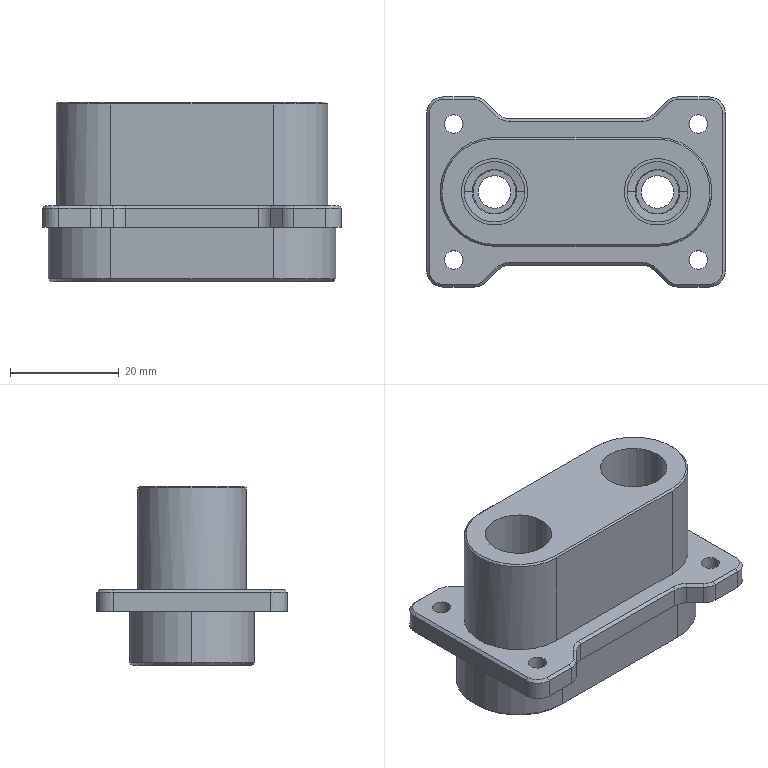NC program | NX | posted with a generic post | part box 55 x 35 x 33 mm
Whole program:
N10 G17 G21 G94 G90
(PLANAR_MILL_6 , TOOL : D6开粗)
N12 T02 M6
N14 G54
N16 G17 G0 G90 X-0.05 Y-1.639 S6500 M3
N18 G43 Z30. H2
N20 Z1.
N22 G94 G1 Y-15.051 Z0.297 F2000.
N24 X0.05 Z0.292
N26 Y-0.001 Z-0.497
N28 Y14.999
N30 X0. Y15.074
N32 X-0.05 Y14.999
N34 Y-15.001
N36 X0. Y-15.076
N38 X0.05 Y-15.001
N40 Y-0.001
N42 X4.25
N44 Y14.999
N46 G3 X0. Y19.249 R4.25
N48 X-4.25 Y14.999 R4.25
N50 G1 Y-15.001
N52 G3 X0. Y-19.251 R4.25
N54 X4.25 Y-15.001 R4.25
N56 G1 Y-0.001
N58 X8.45
N60 Y14.999
N62 G3 X0. Y23.449 R8.45
N64 X-8.45 Y14.999 R8.45
N66 G1 Y-15.001
N68 G3 X0. Y-23.451 R8.45
N70 X8.45 Y-15.001 R8.45
N72 G1 Y-0.001
N74 Z0.503
N76 G0 Z30.
N78 X-0.05 Y-1.639
N80 Z0.503
N82 G1 Y-15.051 Z-0.2
N84 X0.05 Z-0.205
N86 Y-0.001 Z-0.994
N88 Y14.999
N90 X0. Y15.074
N92 X-0.05 Y14.999
N94 Y-15.001
N96 X0. Y-15.076
N98 X0.05 Y-15.001
N100 Y-0.001
N102 X4.25
N104 Y14.999
N106 G3 X0. Y19.249 R4.25
N108 X-4.25 Y14.999 R4.25
N110 G1 Y-15.001
N112 G3 X0. Y-19.251 R4.25
N114 X4.25 Y-15.001 R4.25
N116 G1 Y-0.001
N118 X8.45
N120 Y14.999
N122 G3 X0. Y23.449 R8.45
N124 X-8.45 Y14.999 R8.45
N126 G1 Y-15.001
N128 G3 X0. Y-23.451 R8.45
N130 X8.45 Y-15.001 R8.45
N132 G1 Y-0.001
N134 Z0.006
N136 G0 Z30.
N138 X-0.05 Y-1.639
N140 Z0.006
N142 G1 Y-15.051 Z-0.697
N144 X0.05 Z-0.702
N146 Y-0.001 Z-1.491
N148 Y14.999
N150 X0. Y15.074
N152 X-0.05 Y14.999
N154 Y-15.001
N156 X0. Y-15.076
N158 X0.05 Y-15.001
N160 Y-0.001
N162 X4.25
N164 Y14.999
N166 G3 X0. Y19.249 R4.25
N168 X-4.25 Y14.999 R4.25
N170 G1 Y-15.001
N172 G3 X0. Y-19.251 R4.25
N174 X4.25 Y-15.001 R4.25
N176 G1 Y-0.001
N178 X8.45
N180 Y14.999
N182 G3 X0. Y23.449 R8.45
N184 X-8.45 Y14.999 R8.45
N186 G1 Y-15.001
N188 G3 X0. Y-23.451 R8.45
N190 X8.45 Y-15.001 R8.45
N192 G1 Y-0.001
N194 Z-0.491
N196 G0 Z30.
N198 X-0.05 Y-1.639
N200 Z-0.491
N202 G1 Y-15.051 Z-1.194
N204 X0.05 Z-1.199
N206 Y-0.001 Z-1.988
N208 Y14.999
N210 X0. Y15.074
N212 X-0.05 Y14.999
N214 Y-15.001
N216 X0. Y-15.076
N218 X0.05 Y-15.001
N220 Y-0.001
N222 X4.25
N224 Y14.999
N226 G3 X0. Y19.249 R4.25
N228 X-4.25 Y14.999 R4.25
N230 G1 Y-15.001
N232 G3 X0. Y-19.251 R4.25
N234 X4.25 Y-15.001 R4.25
N236 G1 Y-0.001
N238 X8.45
N240 Y14.999
N242 G3 X0. Y23.449 R8.45
N244 X-8.45 Y14.999 R8.45
N246 G1 Y-15.001
N248 G3 X0. Y-23.451 R8.45
N250 X8.45 Y-15.001 R8.45
N252 G1 Y-0.001
N254 Z-0.988
N256 G0 Z30.
N258 X-0.05 Y-1.639
N260 Z-0.988
N262 G1 Y-15.051 Z-1.69
N264 X0.05 Z-1.696
N266 Y-0.001 Z-2.484
N268 Y14.999
N270 X0. Y15.074
N272 X-0.05 Y14.999
N274 Y-15.001
N276 X0. Y-15.076
N278 X0.05 Y-15.001
N280 Y-0.001
N282 X4.25
N284 Y14.999
N286 G3 X0. Y19.249 R4.25
N288 X-4.25 Y14.999 R4.25
N290 G1 Y-15.001
N292 G3 X0. Y-19.251 R4.25
N294 X4.25 Y-15.001 R4.25
N296 G1 Y-0.001
N298 X8.45
N300 Y14.999
N302 G3 X0. Y23.449 R8.45
N304 X-8.45 Y14.999 R8.45
N306 G1 Y-15.001
N308 G3 X0. Y-23.451 R8.45
N310 X8.45 Y-15.001 R8.45
N312 G1 Y-0.001
N314 Z-1.484
N316 G0 Z30.
N318 X-0.05 Y-1.639
N320 Z-1.484
N322 G1 Y-15.051 Z-2.187
N324 X0.05 Z-2.193
N326 Y-0.001 Z-2.981
N328 Y14.999
N330 X0. Y15.074
N332 X-0.05 Y14.999
N334 Y-15.001
N336 X0. Y-15.076
N338 X0.05 Y-15.001
N340 Y-0.001
N342 X4.25
N344 Y14.999
N346 G3 X0. Y19.249 R4.25
N348 X-4.25 Y14.999 R4.25
N350 G1 Y-15.001
N352 G3 X0. Y-19.251 R4.25
N354 X4.25 Y-15.001 R4.25
N356 G1 Y-0.001
N358 X8.45
N360 Y14.999
N362 G3 X0. Y23.449 R8.45
N364 X-8.45 Y14.999 R8.45
N366 G1 Y-15.001
N368 G3 X0. Y-23.451 R8.45
N370 X8.45 Y-15.001 R8.45
N372 G1 Y-0.001
N374 Z-1.981
N376 G0 Z30.
N378 X-0.05 Y-1.639
N380 Z-1.981
N382 G1 Y-15.051 Z-2.684
N384 X0.05 Z-2.689
N386 Y-0.001 Z-3.478
N388 Y14.999
N390 X0. Y15.074
N392 X-0.05 Y14.999
N394 Y-15.001
N396 X0. Y-15.076
N398 X0.05 Y-15.001
N400 Y-0.001
N402 X4.25
N404 Y14.999
N406 G3 X0. Y19.249 R4.25
N408 X-4.25 Y14.999 R4.25
N410 G1 Y-15.001
N412 G3 X0. Y-19.251 R4.25
N414 X4.25 Y-15.001 R4.25
N416 G1 Y-0.001
N418 X8.45
N420 Y14.999
N422 G3 X0. Y23.449 R8.45
N424 X-8.45 Y14.999 R8.45
N426 G1 Y-15.001
N428 G3 X0. Y-23.451 R8.45
N430 X8.45 Y-15.001 R8.45
N432 G1 Y-0.001
N434 Z-2.478
N436 G0 Z30.
N438 X-0.05 Y-1.639
N440 Z-2.478
N442 G1 Y-15.051 Z-3.181
N444 X0.05 Z-3.186
N446 Y-0.001 Z-3.975
N448 Y14.999
N450 X0. Y15.074
N452 X-0.05 Y14.999
N454 Y-15.001
N456 X0. Y-15.076
N458 X0.05 Y-15.001
N460 Y-0.001
N462 X4.25
N464 Y14.999
N466 G3 X0. Y19.249 R4.25
N468 X-4.25 Y14.999 R4.25
N470 G1 Y-15.001
N472 G3 X0. Y-19.251 R4.25
N474 X4.25 Y-15.001 R4.25
N476 G1 Y-0.001
N478 X8.45
N480 Y14.999
N482 G3 X0. Y23.449 R8.45
N484 X-8.45 Y14.999 R8.45
N486 G1 Y-15.001
N488 G3 X0. Y-23.451 R8.45
N490 X8.45 Y-15.001 R8.45
N492 G1 Y-0.001
N494 Z-2.975
N496 G0 Z30.
N498 X-0.05 Y-1.639
N500 Z-2.975
N502 G1 Y-15.051 Z-3.678
N504 X0.05 Z-3.683
N506 Y-0.001 Z-4.472
N508 Y14.999
N510 X0. Y15.074
N512 X-0.05 Y14.999
N514 Y-15.001
N516 X0. Y-15.076
N518 X0.05 Y-15.001
N520 Y-0.001
N522 X4.25
N524 Y14.999
N526 G3 X0. Y19.249 R4.25
N528 X-4.25 Y14.999 R4.25
N530 G1 Y-15.001
N532 G3 X0. Y-19.251 R4.25
N534 X4.25 Y-15.001 R4.25
N536 G1 Y-0.001
N538 X8.45
N540 Y14.999
N542 G3 X0. Y23.449 R8.45
N544 X-8.45 Y14.999 R8.45
N546 G1 Y-15.001
N548 G3 X0. Y-23.451 R8.45
N550 X8.45 Y-15.001 R8.45
N552 G1 Y-0.001
N554 Z-3.472
N556 G0 Z30.
N558 X-0.05 Y-1.639
N560 Z-3.472
N562 G1 Y-15.051 Z-4.175
N564 X0.05 Z-4.18
N566 Y-0.001 Z-4.969
N568 Y14.999
N570 X0. Y15.074
N572 X-0.05 Y14.999
N574 Y-15.001
N576 X0. Y-15.076
N578 X0.05 Y-15.001
N580 Y-0.001
N582 X4.25
N584 Y14.999
N586 G3 X0. Y19.249 R4.25
N588 X-4.25 Y14.999 R4.25
N590 G1 Y-15.001
N592 G3 X0. Y-19.251 R4.25
N594 X4.25 Y-15.001 R4.25
N596 G1 Y-0.001
N598 X8.45
N600 Y14.999
N602 G3 X0. Y23.449 R8.45
N604 X-8.45 Y14.999 R8.45
N606 G1 Y-15.001
N608 G3 X0. Y-23.451 R8.45
N610 X8.45 Y-15.001 R8.45
N612 G1 Y-0.001
N614 Z-3.969
N616 G0 Z30.
N618 X-0.05 Y-1.639
N620 Z-3.969
N622 G1 Y-15.051 Z-4.672
N624 X0.05 Z-4.677
N626 Y-0.001 Z-5.466
N628 Y14.999
N630 X0. Y15.074
N632 X-0.05 Y14.999
N634 Y-15.001
N636 X0. Y-15.076
N638 X0.05 Y-15.001
N640 Y-0.001
N642 X4.25
N644 Y14.999
N646 G3 X0. Y19.249 R4.25
N648 X-4.25 Y14.999 R4.25
N650 G1 Y-15.001
N652 G3 X0. Y-19.251 R4.25
N654 X4.25 Y-15.001 R4.25
N656 G1 Y-0.001
N658 X8.45
N660 Y14.999
N662 G3 X0. Y23.449 R8.45
N664 X-8.45 Y14.999 R8.45
N666 G1 Y-15.001
N668 G3 X0. Y-23.451 R8.45
N670 X8.45 Y-15.001 R8.45
N672 G1 Y-0.001
N674 Z-4.466
N676 G0 Z30.
N678 X-0.05 Y-1.639
N680 Z-4.466
N682 G1 Y-15.051 Z-5.169
N684 X0.05 Z-5.174
N686 Y-0.001 Z-5.963
N688 Y14.999
N690 X0. Y15.074
N692 X-0.05 Y14.999
N694 Y-15.001
N696 X0. Y-15.076
N698 X0.05 Y-15.001
N700 Y-0.001
N702 X4.25
N704 Y14.999
N706 G3 X0. Y19.249 R4.25
N708 X-4.25 Y14.999 R4.25
N710 G1 Y-15.001
N712 G3 X0. Y-19.251 R4.25
N714 X4.25 Y-15.001 R4.25
N716 G1 Y-0.001
N718 X8.45
N720 Y14.999
N722 G3 X0. Y23.449 R8.45
N724 X-8.45 Y14.999 R8.45
N726 G1 Y-15.001
N728 G3 X0. Y-23.451 R8.45
N730 X8.45 Y-15.001 R8.45
N732 G1 Y-0.001
N734 Z-4.963
N736 G0 Z30.
N738 X-0.05 Y-1.639
N740 Z-4.963
N742 G1 Y-15.051 Z-5.665
N744 X0.05 Z-5.671
N746 Y-0.001 Z-6.459
N748 Y14.999
N750 X0. Y15.074
N752 X-0.05 Y14.999
N754 Y-15.001
N756 X0. Y-15.076
N758 X0.05 Y-15.001
N760 Y-0.001
N762 X4.25
N764 Y14.999
N766 G3 X0. Y19.249 R4.25
N768 X-4.25 Y14.999 R4.25
N770 G1 Y-15.001
N772 G3 X0. Y-19.251 R4.25
N774 X4.25 Y-15.001 R4.25
N776 G1 Y-0.001
N778 X8.45
N780 Y14.999
N782 G3 X0. Y23.449 R8.45
N784 X-8.45 Y14.999 R8.45
N786 G1 Y-15.001
N788 G3 X0. Y-23.451 R8.45
N790 X8.45 Y-15.001 R8.45
N792 G1 Y-0.001
N794 Z-5.459
N796 G0 Z30.
N798 X-0.05 Y-1.639
N800 Z-5.459
N802 G1 Y-15.051 Z-6.162
N804 X0.05 Z-6.168
N806 Y-0.001 Z-6.956
N808 Y14.999
N810 X0. Y15.074
N812 X-0.05 Y14.999
N814 Y-15.001
N816 X0. Y-15.076
N818 X0.05 Y-15.001
N820 Y-0.001
N822 X4.25
N824 Y14.999
N826 G3 X0. Y19.249 R4.25
N828 X-4.25 Y14.999 R4.25
N830 G1 Y-15.001
N832 G3 X0. Y-19.251 R4.25
N834 X4.25 Y-15.001 R4.25
N836 G1 Y-0.001
N838 X8.45
N840 Y14.999
N842 G3 X0. Y23.449 R8.45
N844 X-8.45 Y14.999 R8.45
N846 G1 Y-15.001
N848 G3 X0. Y-23.451 R8.45
N850 X8.45 Y-15.001 R8.45
N852 G1 Y-0.001
N854 Z-5.956
N856 G0 Z30.
N858 X-0.05 Y-1.639
N860 Z-5.956
N862 G1 Y-15.051 Z-6.659
N864 X0.05 Z-6.664
N866 Y-0.001 Z-7.453
N868 Y14.999
N870 X0. Y15.074
N872 X-0.05 Y14.999
N874 Y-15.001
N876 X0. Y-15.076
N878 X0.05 Y-15.001
N880 Y-0.001
N882 X4.25
N884 Y14.999
N886 G3 X0. Y19.249 R4.25
N888 X-4.25 Y14.999 R4.25
N890 G1 Y-15.001
N892 G3 X0. Y-19.251 R4.25
N894 X4.25 Y-15.001 R4.25
N896 G1 Y-0.001
N898 X8.45
N900 Y14.999
N902 G3 X0. Y23.449 R8.45
N904 X-8.45 Y14.999 R8.45
N906 G1 Y-15.001
N908 G3 X0. Y-23.451 R8.45
N910 X8.45 Y-15.001 R8.45
N912 G1 Y-0.001
N914 Z-6.453
N916 G0 Z30.
N918 X-0.05 Y-1.639
N920 Z-6.453
N922 G1 Y-15.051 Z-7.156
N924 X0.05 Z-7.161
N926 Y-0.001 Z-7.95
N928 Y14.999
N930 X0. Y15.074
N932 X-0.05 Y14.999
N934 Y-15.001
N936 X0. Y-15.076
N938 X0.05 Y-15.001
N940 Y-0.001
N942 X4.25
N944 Y14.999
N946 G3 X0. Y19.249 R4.25
N948 X-4.25 Y14.999 R4.25
N950 G1 Y-15.001
N952 G3 X0. Y-19.251 R4.25
N954 X4.25 Y-15.001 R4.25
N956 G1 Y-0.001
N958 X8.45
N960 Y14.999
N962 G3 X0. Y23.449 R8.45
N964 X-8.45 Y14.999 R8.45
N966 G1 Y-15.001
N968 G3 X0. Y-23.451 R8.45
N970 X8.45 Y-15.001 R8.45
N972 G1 Y-0.001
N974 Z-6.95
N976 G0 Z30.
(PLANAR_MILL_6_COPY , TOOL : D6开粗)
N978 X-0.05 Y-11.12
N980 Z-7.
N982 G1 Y-15.051 Z-7.206 F800.
N984 X0.05 Z-7.211
N986 Y-0.001 Z-8.
N988 Y14.999
N990 X0. Y15.074
N992 X-0.05 Y14.999
N994 Y-15.001
N996 X0. Y-15.076
N998 X0.05 Y-15.001
N1000 Y-0.001
N1002 X4.25
N1004 Y14.999
N1006 G3 X0. Y19.249 R4.25
N1008 X-4.25 Y14.999 R4.25
N1010 G1 Y-15.001
N1012 G3 X0. Y-19.251 R4.25
N1014 X4.25 Y-15.001 R4.25
N1016 G1 Y-0.001
N1018 X8.45
N1020 Y14.999
N1022 G3 X0. Y23.449 R8.45
N1024 X-8.45 Y14.999 R8.45
N1026 G1 Y-15.001
N1028 G3 X0. Y-23.451 R8.45
N1030 X8.45 Y-15.001 R8.45
N1032 G1 Y-0.001
N1034 Z-7.
N1036 G0 Z30.
(PLANAR_MILL_6_COPY_COPY , TOOL : D6开粗)
N1038 X7.303 Y-0.967
N1040 Z-6.
N1042 G1 Z-8.
N1044 G41 X7.5 Y-1.001 D2
N1046 G3 X8.5 Y-0.001 R1.
N1048 G1 Y14.999
N1050 G3 X0. Y23.499 R8.5
N1052 X-8.5 Y14.999 R8.5
N1054 G1 Y-15.001
N1056 G3 X0. Y-23.501 R8.5
N1058 X8.5 Y-15.001 R8.5
N1060 G1 Y-0.001
N1062 G3 X7.5 Y0.999 R1.
N1064 G40
N1066 G1 X7.303 Y0.964
N1068 Z-6.
N1070 G0 Z30.
N1072 M5
N1074 M2